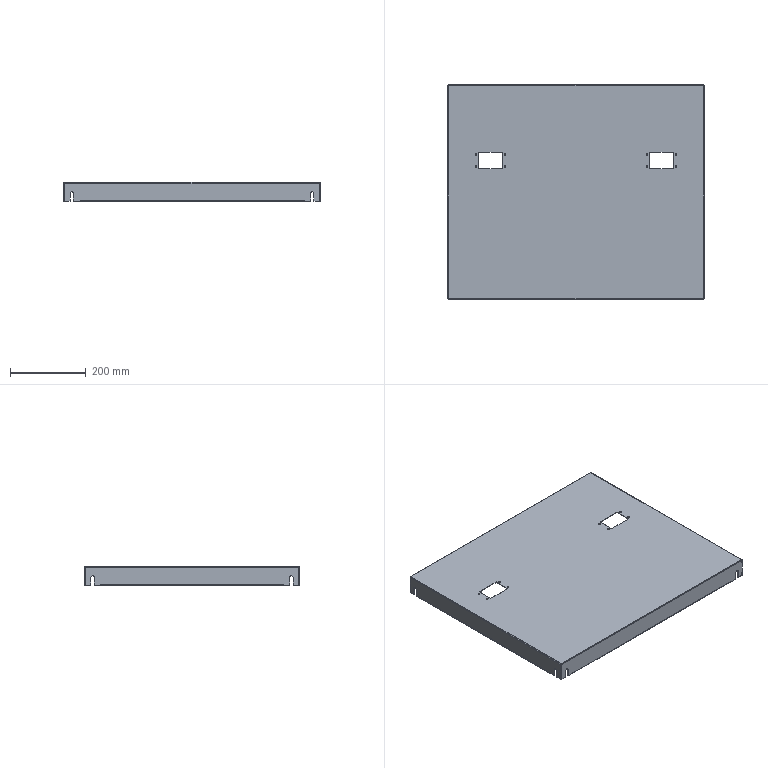Part | SolidWorks | features BaseBody 1 | 1 solid | 174 faces | box 675 x 565 x 51.5 mm | volume 767845 mm3 | plane 110 | cylinder 56 | spline 8 | commonest cylinder face diameters 4.5 x16 9 x16 1.473 x8 4.473 x8 6 x8